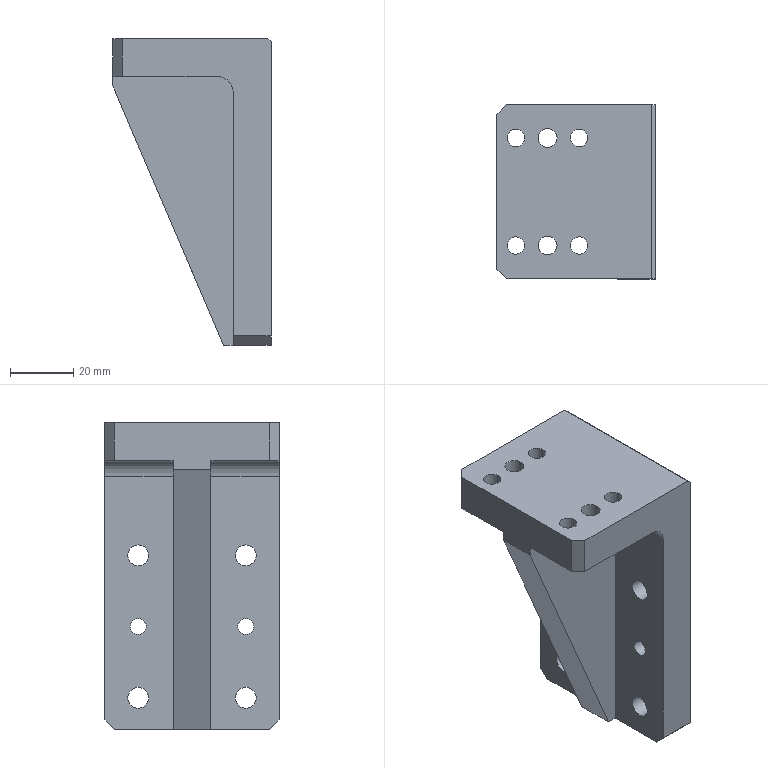Part | NX | 1 solid | 32 faces | box 50 x 55 x 97 mm | volume 106695 mm3 | plane 18 | cylinder 14 | commonest cylinder face diameters 5.5 x4 6.6 x4 5 x2 6 x2 10 x2
STEP:
#1=CARTESIAN_POINT('',(24.,55.,48.5));
#2=VERTEX_POINT('',#1);
#3=CARTESIAN_POINT('',(25.,55.,47.5));
#4=VERTEX_POINT('',#3);
#5=CARTESIAN_POINT('',(25.,55.,47.5));
#6=DIRECTION('',(0.7071,0.,-0.7071));
#7=VECTOR('',#6,1000.);
#8=LINE('',#5,#7);
#9=EDGE_CURVE('',#2,#4,#8,.T.);
#10=ORIENTED_EDGE('',*,*,#9,.F.);
#11=CARTESIAN_POINT('',(24.,0.,48.5));
#12=VERTEX_POINT('',#11);
#13=CARTESIAN_POINT('',(24.,55.,48.5));
#14=DIRECTION('',(0.,1.,0.));
#15=VECTOR('',#14,1000.);
#16=LINE('',#13,#15);
#17=EDGE_CURVE('',#12,#2,#16,.T.);
#18=ORIENTED_EDGE('',*,*,#17,.F.);
#19=CARTESIAN_POINT('',(25.,0.,47.5));
#20=VERTEX_POINT('',#19);
#21=CARTESIAN_POINT('',(36.25,0.,36.25));
#22=DIRECTION('',(-0.7071,0.,0.7071));
#23=VECTOR('',#22,1000.);
#24=LINE('',#21,#23);
#25=EDGE_CURVE('',#20,#12,#24,.T.);
#26=ORIENTED_EDGE('',*,*,#25,.F.);
#27=CARTESIAN_POINT('',(25.,55.,47.5));
#28=DIRECTION('',(0.,-1.,0.));
#29=VECTOR('',#28,1000.);
#30=LINE('',#27,#29);
#31=EDGE_CURVE('',#4,#20,#30,.T.);
#32=ORIENTED_EDGE('',*,*,#31,.F.);
#33=EDGE_LOOP('',(#10,#18,#26,#32));
#34=FACE_BOUND('',#33,.T.);
#35=CARTESIAN_POINT('',(25.,55.,47.5));
#36=DIRECTION('',(-0.7071,0.,-0.7071));
#37=DIRECTION('',(0.,-1.,0.));
#38=AXIS2_PLACEMENT_3D('',#35,#36,#37);
#39=PLANE('',#38);
#40=ADVANCED_FACE('',(#34),#39,.F.);
#41=CARTESIAN_POINT('',(25.,52.,-48.5));
#42=VERTEX_POINT('',#41);
#43=CARTESIAN_POINT('',(25.,55.,-45.5));
#44=VERTEX_POINT('',#43);
#45=CARTESIAN_POINT('',(25.,55.,-45.5));
#46=DIRECTION('',(0.,0.7071,0.7071));
#47=VECTOR('',#46,1000.);
#48=LINE('',#45,#47);
#49=EDGE_CURVE('',#42,#44,#48,.T.);
#50=ORIENTED_EDGE('',*,*,#49,.F.);
#51=CARTESIAN_POINT('',(13.,52.,-48.5));
#52=VERTEX_POINT('',#51);
#53=CARTESIAN_POINT('',(-25.,52.,-48.5));
#54=DIRECTION('',(1.,0.,0.));
#55=VECTOR('',#54,1000.);
#56=LINE('',#53,#55);
#57=EDGE_CURVE('',#52,#42,#56,.T.);
#58=ORIENTED_EDGE('',*,*,#57,.F.);
#59=CARTESIAN_POINT('',(13.,55.,-45.5));
#60=VERTEX_POINT('',#59);
#61=CARTESIAN_POINT('',(13.,55.,-45.5));
#62=DIRECTION('',(0.,-0.7071,-0.7071));
#63=VECTOR('',#62,1000.);
#64=LINE('',#61,#63);
#65=EDGE_CURVE('',#60,#52,#64,.T.);
#66=ORIENTED_EDGE('',*,*,#65,.F.);
#67=CARTESIAN_POINT('',(0.,55.,-45.5));
#68=DIRECTION('',(-1.,0.,0.));
#69=VECTOR('',#68,1000.);
#70=LINE('',#67,#69);
#71=EDGE_CURVE('',#44,#60,#70,.T.);
#72=ORIENTED_EDGE('',*,*,#71,.F.);
#73=EDGE_LOOP('',(#50,#58,#66,#72));
#74=FACE_BOUND('',#73,.T.);
#75=CARTESIAN_POINT('',(0.,55.,-45.5));
#76=DIRECTION('',(0.,-0.7071,0.7071));
#77=DIRECTION('',(-1.,0.,0.));
#78=AXIS2_PLACEMENT_3D('',#75,#76,#77);
#79=PLANE('',#78);
#80=ADVANCED_FACE('',(#74),#79,.F.);
#81=CARTESIAN_POINT('',(-25.,52.,36.5));
#82=VERTEX_POINT('',#81);
#83=CARTESIAN_POINT('',(-22.,55.,36.5));
#84=VERTEX_POINT('',#83);
#85=CARTESIAN_POINT('',(-22.,55.,36.5));
#86=DIRECTION('',(0.7071,0.7071,0.));
#87=VECTOR('',#86,1000.);
#88=LINE('',#85,#87);
#89=EDGE_CURVE('',#82,#84,#88,.T.);
#90=ORIENTED_EDGE('',*,*,#89,.F.);
#91=CARTESIAN_POINT('',(-25.,52.,48.5));
#92=VERTEX_POINT('',#91);
#93=CARTESIAN_POINT('',(-25.,52.,48.5));
#94=DIRECTION('',(0.,0.,-1.));
#95=VECTOR('',#94,1000.);
#96=LINE('',#93,#95);
#97=EDGE_CURVE('',#92,#82,#96,.T.);
#98=ORIENTED_EDGE('',*,*,#97,.F.);
#99=CARTESIAN_POINT('',(-22.,55.,48.5));
#100=VERTEX_POINT('',#99);
#101=CARTESIAN_POINT('',(-22.,55.,48.5));
#102=DIRECTION('',(-0.7071,-0.7071,0.));
#103=VECTOR('',#102,1000.);
#104=LINE('',#101,#103);
#105=EDGE_CURVE('',#100,#92,#104,.T.);
#106=ORIENTED_EDGE('',*,*,#105,.F.);
#107=CARTESIAN_POINT('',(-22.,55.,0.));
#108=DIRECTION('',(0.,0.,1.));
#109=VECTOR('',#108,1000.);
#110=LINE('',#107,#109);
#111=EDGE_CURVE('',#84,#100,#110,.T.);
#112=ORIENTED_EDGE('',*,*,#111,.F.);
#113=EDGE_LOOP('',(#90,#98,#106,#112));
#114=FACE_BOUND('',#113,.T.);
#115=CARTESIAN_POINT('',(-22.,55.,0.));
#116=DIRECTION('',(0.7071,-0.7071,0.));
#117=DIRECTION('',(0.,0.,1.));
#118=AXIS2_PLACEMENT_3D('',#115,#116,#117);
#119=PLANE('',#118);
#120=ADVANCED_FACE('',(#114),#119,.F.);
#121=CARTESIAN_POINT('',(25.,0.,-45.5));
#122=VERTEX_POINT('',#121);
#123=CARTESIAN_POINT('',(25.,3.,-48.5));
#124=VERTEX_POINT('',#123);
#125=CARTESIAN_POINT('',(25.,3.,-48.5));
#126=DIRECTION('',(0.,0.7071,-0.7071));
#127=VECTOR('',#126,1000.);
#128=LINE('',#125,#127);
#129=EDGE_CURVE('',#122,#124,#128,.T.);
#130=ORIENTED_EDGE('',*,*,#129,.F.);
#131=CARTESIAN_POINT('',(13.,0.,-45.5));
#132=VERTEX_POINT('',#131);
#133=CARTESIAN_POINT('',(25.,0.,-45.5));
#134=DIRECTION('',(1.,0.,0.));
#135=VECTOR('',#134,1000.);
#136=LINE('',#133,#135);
#137=EDGE_CURVE('',#132,#122,#136,.T.);
#138=ORIENTED_EDGE('',*,*,#137,.F.);
#139=CARTESIAN_POINT('',(13.,3.,-48.5));
#140=VERTEX_POINT('',#139);
#141=CARTESIAN_POINT('',(13.,18.25,-63.75));
#142=DIRECTION('',(0.,-0.7071,0.7071));
#143=VECTOR('',#142,1000.);
#144=LINE('',#141,#143);
#145=EDGE_CURVE('',#140,#132,#144,.T.);
#146=ORIENTED_EDGE('',*,*,#145,.F.);
#147=CARTESIAN_POINT('',(13.,3.,-48.5));
#148=DIRECTION('',(-1.,0.,0.));
#149=VECTOR('',#148,1000.);
#150=LINE('',#147,#149);
#151=EDGE_CURVE('',#124,#140,#150,.T.);
#152=ORIENTED_EDGE('',*,*,#151,.F.);
#153=EDGE_LOOP('',(#130,#138,#146,#152));
#154=FACE_BOUND('',#153,.T.);
#155=CARTESIAN_POINT('',(-25.,3.,-48.5));
#156=DIRECTION('',(0.,-0.7071,-0.7071));
#157=DIRECTION('',(1.,0.,0.));
#158=AXIS2_PLACEMENT_3D('',#155,#156,#157);
#159=PLANE('',#158);
#160=ADVANCED_FACE('',(#154),#159,.T.);
#161=CARTESIAN_POINT('',(-22.,0.,36.5));
#162=VERTEX_POINT('',#161);
#163=CARTESIAN_POINT('',(-25.,3.,36.5));
#164=VERTEX_POINT('',#163);
#165=CARTESIAN_POINT('',(-21.25,-0.75,36.5));
#166=DIRECTION('',(-0.7071,0.7071,0.));
#167=VECTOR('',#166,1000.);
#168=LINE('',#165,#167);
#169=EDGE_CURVE('',#162,#164,#168,.T.);
#170=ORIENTED_EDGE('',*,*,#169,.F.);
#171=CARTESIAN_POINT('',(-22.,0.,48.5));
#172=VERTEX_POINT('',#171);
#173=CARTESIAN_POINT('',(-22.,0.,36.5));
#174=DIRECTION('',(0.,0.,-1.));
#175=VECTOR('',#174,1000.);
#176=LINE('',#173,#175);
#177=EDGE_CURVE('',#172,#162,#176,.T.);
#178=ORIENTED_EDGE('',*,*,#177,.F.);
#179=CARTESIAN_POINT('',(-25.,3.,48.5));
#180=VERTEX_POINT('',#179);
#181=CARTESIAN_POINT('',(-25.,3.,48.5));
#182=DIRECTION('',(0.7071,-0.7071,0.));
#183=VECTOR('',#182,1000.);
#184=LINE('',#181,#183);
#185=EDGE_CURVE('',#180,#172,#184,.T.);
#186=ORIENTED_EDGE('',*,*,#185,.F.);
#187=CARTESIAN_POINT('',(-25.,3.,48.5));
#188=DIRECTION('',(0.,0.,1.));
#189=VECTOR('',#188,1000.);
#190=LINE('',#187,#189);
#191=EDGE_CURVE('',#164,#180,#190,.T.);
#192=ORIENTED_EDGE('',*,*,#191,.F.);
#193=EDGE_LOOP('',(#170,#178,#186,#192));
#194=FACE_BOUND('',#193,.T.);
#195=CARTESIAN_POINT('',(-25.,3.,48.5));
#196=DIRECTION('',(-0.7071,-0.7071,0.));
#197=DIRECTION('',(0.,0.,-1.));
#198=AXIS2_PLACEMENT_3D('',#195,#196,#197);
#199=PLANE('',#198);
#200=ADVANCED_FACE('',(#194),#199,.T.);
#201=CARTESIAN_POINT('',(8.,33.5,36.5));
#202=VERTEX_POINT('',#201);
#203=CARTESIAN_POINT('',(13.,33.5,31.5));
#204=VERTEX_POINT('',#203);
#205=CARTESIAN_POINT('',(8.,33.5,31.5));
#206=DIRECTION('',(0.,1.,0.));
#207=DIRECTION('',(0.,0.,1.));
#208=AXIS2_PLACEMENT_3D('',#205,#206,#207);
#209=CIRCLE('',#208,5.);
#210=EDGE_CURVE('',#202,#204,#209,.T.);
#211=ORIENTED_EDGE('',*,*,#210,.F.);
#212=CARTESIAN_POINT('',(8.,55.,36.5));
#213=VERTEX_POINT('',#212);
#214=CARTESIAN_POINT('',(8.,33.5,36.5));
#215=DIRECTION('',(0.,-1.,0.));
#216=VECTOR('',#215,1000.);
#217=LINE('',#214,#216);
#218=EDGE_CURVE('',#213,#202,#217,.T.);
#219=ORIENTED_EDGE('',*,*,#218,.F.);
#220=CARTESIAN_POINT('',(13.,55.,31.5));
#221=VERTEX_POINT('',#220);
#222=CARTESIAN_POINT('',(8.,55.,31.5));
#223=DIRECTION('',(0.,-1.,0.));
#224=DIRECTION('',(0.,0.,-1.));
#225=AXIS2_PLACEMENT_3D('',#222,#223,#224);
#226=CIRCLE('',#225,5.);
#227=EDGE_CURVE('',#221,#213,#226,.T.);
#228=ORIENTED_EDGE('',*,*,#227,.F.);
#229=CARTESIAN_POINT('',(13.,55.,31.5));
#230=DIRECTION('',(0.,1.,0.));
#231=VECTOR('',#230,1000.);
#232=LINE('',#229,#231);
#233=EDGE_CURVE('',#204,#221,#232,.T.);
#234=ORIENTED_EDGE('',*,*,#233,.F.);
#235=EDGE_LOOP('',(#211,#219,#228,#234));
#236=FACE_BOUND('',#235,.T.);
#237=CARTESIAN_POINT('',(8.,33.5,31.5));
#238=DIRECTION('',(0.,-1.,0.));
#239=DIRECTION('',(0.,0.,-1.));
#240=AXIS2_PLACEMENT_3D('',#237,#238,#239);
#241=CYLINDRICAL_SURFACE('',#240,5.);
#242=ADVANCED_FACE('',(#236),#241,.F.);
#243=CARTESIAN_POINT('',(13.,21.5,31.5));
#244=VERTEX_POINT('',#243);
#245=CARTESIAN_POINT('',(8.,21.5,36.5));
#246=VERTEX_POINT('',#245);
#247=CARTESIAN_POINT('',(8.,21.5,31.5));
#248=DIRECTION('',(0.,-1.,0.));
#249=DIRECTION('',(0.,0.,-1.));
#250=AXIS2_PLACEMENT_3D('',#247,#248,#249);
#251=CIRCLE('',#250,5.);
#252=EDGE_CURVE('',#244,#246,#251,.T.);
#253=ORIENTED_EDGE('',*,*,#252,.F.);
#254=CARTESIAN_POINT('',(13.,0.,31.5));
#255=VERTEX_POINT('',#254);
#256=CARTESIAN_POINT('',(13.,21.5,31.5));
#257=DIRECTION('',(0.,1.,0.));
#258=VECTOR('',#257,1000.);
#259=LINE('',#256,#258);
#260=EDGE_CURVE('',#255,#244,#259,.T.);
#261=ORIENTED_EDGE('',*,*,#260,.F.);
#262=CARTESIAN_POINT('',(8.,0.,36.5));
#263=VERTEX_POINT('',#262);
#264=CARTESIAN_POINT('',(8.,0.,31.5));
#265=DIRECTION('',(0.,1.,0.));
#266=DIRECTION('',(0.,0.,-1.));
#267=AXIS2_PLACEMENT_3D('',#264,#265,#266);
#268=CIRCLE('',#267,5.);
#269=EDGE_CURVE('',#263,#255,#268,.T.);
#270=ORIENTED_EDGE('',*,*,#269,.F.);
#271=CARTESIAN_POINT('',(8.,21.5,36.5));
#272=DIRECTION('',(0.,-1.,0.));
#273=VECTOR('',#272,1000.);
#274=LINE('',#271,#273);
#275=EDGE_CURVE('',#246,#263,#274,.T.);
#276=ORIENTED_EDGE('',*,*,#275,.F.);
#277=EDGE_LOOP('',(#253,#261,#270,#276));
#278=FACE_BOUND('',#277,.T.);
#279=CARTESIAN_POINT('',(8.,21.5,31.5));
#280=DIRECTION('',(0.,1.,0.));
#281=DIRECTION('',(0.,0.,1.));
#282=AXIS2_PLACEMENT_3D('',#279,#280,#281);
#283=CYLINDRICAL_SURFACE('',#282,5.);
#284=ADVANCED_FACE('',(#278),#283,.F.);
#285=CARTESIAN_POINT('',(13.,21.5,-48.5));
#286=VERTEX_POINT('',#285);
#287=CARTESIAN_POINT('',(13.,21.5,-48.5));
#288=DIRECTION('',(0.,0.,-1.));
#289=VECTOR('',#288,1000.);
#290=LINE('',#287,#289);
#291=EDGE_CURVE('',#244,#286,#290,.T.);
#292=ORIENTED_EDGE('',*,*,#291,.F.);
#293=ORIENTED_EDGE('',*,*,#252,.T.);
#294=CARTESIAN_POINT('',(-25.,21.5,36.5));
#295=VERTEX_POINT('',#294);
#296=CARTESIAN_POINT('',(13.,21.5,36.5));
#297=DIRECTION('',(1.,0.,0.));
#298=VECTOR('',#297,1000.);
#299=LINE('',#296,#298);
#300=EDGE_CURVE('',#295,#246,#299,.T.);
#301=ORIENTED_EDGE('',*,*,#300,.F.);
#302=CARTESIAN_POINT('',(-25.,21.5,33.5));
#303=VERTEX_POINT('',#302);
#304=CARTESIAN_POINT('',(-25.,21.5,33.5));
#305=DIRECTION('',(0.,0.,1.));
#306=VECTOR('',#305,1000.);
#307=LINE('',#304,#306);
#308=EDGE_CURVE('',#303,#295,#307,.T.);
#309=ORIENTED_EDGE('',*,*,#308,.F.);
#310=CARTESIAN_POINT('',(10.,21.5,-48.5));
#311=VERTEX_POINT('',#310);
#312=CARTESIAN_POINT('',(-25.,21.5,33.5));
#313=DIRECTION('',(-0.3926,0.,0.9197));
#314=VECTOR('',#313,1000.);
#315=LINE('',#312,#314);
#316=EDGE_CURVE('',#311,#303,#315,.T.);
#317=ORIENTED_EDGE('',*,*,#316,.F.);
#318=CARTESIAN_POINT('',(13.,21.5,-48.5));
#319=DIRECTION('',(-1.,0.,0.));
#320=VECTOR('',#319,1000.);
#321=LINE('',#318,#320);
#322=EDGE_CURVE('',#286,#311,#321,.T.);
#323=ORIENTED_EDGE('',*,*,#322,.F.);
#324=EDGE_LOOP('',(#292,#293,#301,#309,#317,#323));
#325=FACE_BOUND('',#324,.T.);
#326=CARTESIAN_POINT('',(0.,21.5,0.));
#327=DIRECTION('',(0.,-1.,0.));
#328=DIRECTION('',(0.,0.,1.));
#329=AXIS2_PLACEMENT_3D('',#326,#327,#328);
#330=PLANE('',#329);
#331=ADVANCED_FACE('',(#325),#330,.T.);
#332=CARTESIAN_POINT('',(13.,33.5,-48.5));
#333=DIRECTION('',(0.,-1.,0.));
#334=VECTOR('',#333,1000.);
#335=LINE('',#332,#334);
#336=EDGE_CURVE('',#286,#140,#335,.T.);
#337=ORIENTED_EDGE('',*,*,#336,.T.);
#338=ORIENTED_EDGE('',*,*,#145,.T.);
#339=CARTESIAN_POINT('',(13.,0.,0.));
#340=DIRECTION('',(0.,0.,-1.));
#341=VECTOR('',#340,1000.);
#342=LINE('',#339,#341);
#343=EDGE_CURVE('',#255,#132,#342,.T.);
#344=ORIENTED_EDGE('',*,*,#343,.F.);
#345=ORIENTED_EDGE('',*,*,#260,.T.);
#346=ORIENTED_EDGE('',*,*,#291,.T.);
#347=EDGE_LOOP('',(#337,#338,#344,#345,#346));
#348=FACE_BOUND('',#347,.T.);
#349=CARTESIAN_POINT('',(13.,10.5,3.2));
#350=VERTEX_POINT('',#349);
#351=CARTESIAN_POINT('',(13.,10.5,6.5));
#352=DIRECTION('',(-1.,0.,0.));
#353=DIRECTION('',(0.,0.,-1.));
#354=AXIS2_PLACEMENT_3D('',#351,#352,#353);
#355=CIRCLE('',#354,3.3);
#356=EDGE_CURVE('',#350,#350,#355,.T.);
#357=ORIENTED_EDGE('',*,*,#356,.F.);
#358=EDGE_LOOP('',(#357));
#359=FACE_BOUND('',#358,.T.);
#360=CARTESIAN_POINT('',(13.,10.5,-41.8));
#361=VERTEX_POINT('',#360);
#362=CARTESIAN_POINT('',(13.,10.5,-38.5));
#363=DIRECTION('',(-1.,0.,0.));
#364=DIRECTION('',(0.,0.,-1.));
#365=AXIS2_PLACEMENT_3D('',#362,#363,#364);
#366=CIRCLE('',#365,3.3);
#367=EDGE_CURVE('',#361,#361,#366,.T.);
#368=ORIENTED_EDGE('',*,*,#367,.F.);
#369=EDGE_LOOP('',(#368));
#370=FACE_BOUND('',#369,.T.);
#371=CARTESIAN_POINT('',(13.,10.5,-18.5));
#372=VERTEX_POINT('',#371);
#373=CARTESIAN_POINT('',(13.,10.5,-16.));
#374=DIRECTION('',(-1.,0.,0.));
#375=DIRECTION('',(0.,0.,-1.));
#376=AXIS2_PLACEMENT_3D('',#373,#374,#375);
#377=CIRCLE('',#376,2.5);
#378=EDGE_CURVE('',#372,#372,#377,.T.);
#379=ORIENTED_EDGE('',*,*,#378,.F.);
#380=EDGE_LOOP('',(#379));
#381=FACE_BOUND('',#380,.T.);
#382=CARTESIAN_POINT('',(13.,33.5,-48.5));
#383=DIRECTION('',(1.,0.,0.));
#384=DIRECTION('',(0.,0.,-1.));
#385=AXIS2_PLACEMENT_3D('',#382,#383,#384);
#386=PLANE('',#385);
#387=ADVANCED_FACE('',(#348,#359,#370,#381),#386,.F.);
#388=CARTESIAN_POINT('',(0.,0.,36.5));
#389=DIRECTION('',(1.,0.,0.));
#390=VECTOR('',#389,1000.);
#391=LINE('',#388,#390);
#392=EDGE_CURVE('',#162,#263,#391,.T.);
#393=ORIENTED_EDGE('',*,*,#392,.F.);
#394=ORIENTED_EDGE('',*,*,#169,.T.);
#395=CARTESIAN_POINT('',(-25.,55.,36.5));
#396=DIRECTION('',(0.,-1.,0.));
#397=VECTOR('',#396,1000.);
#398=LINE('',#395,#397);
#399=EDGE_CURVE('',#295,#164,#398,.T.);
#400=ORIENTED_EDGE('',*,*,#399,.F.);
#401=ORIENTED_EDGE('',*,*,#300,.T.);
#402=ORIENTED_EDGE('',*,*,#275,.T.);
#403=EDGE_LOOP('',(#393,#394,#400,#401,#402));
#404=FACE_BOUND('',#403,.T.);
#405=CARTESIAN_POINT('',(-16.25,10.5,36.5));
#406=VERTEX_POINT('',#405);
#407=CARTESIAN_POINT('',(-19.,10.5,36.5));
#408=DIRECTION('',(0.,0.,-1.));
#409=DIRECTION('',(1.,0.,0.));
#410=AXIS2_PLACEMENT_3D('',#407,#408,#409);
#411=CIRCLE('',#410,2.75);
#412=EDGE_CURVE('',#406,#406,#411,.T.);
#413=ORIENTED_EDGE('',*,*,#412,.F.);
#414=EDGE_LOOP('',(#413));
#415=FACE_BOUND('',#414,.T.);
#416=CARTESIAN_POINT('',(3.75,10.5,36.5));
#417=VERTEX_POINT('',#416);
#418=CARTESIAN_POINT('',(1.,10.5,36.5));
#419=DIRECTION('',(0.,0.,-1.));
#420=DIRECTION('',(1.,0.,0.));
#421=AXIS2_PLACEMENT_3D('',#418,#419,#420);
#422=CIRCLE('',#421,2.75);
#423=EDGE_CURVE('',#417,#417,#422,.T.);
#424=ORIENTED_EDGE('',*,*,#423,.F.);
#425=EDGE_LOOP('',(#424));
#426=FACE_BOUND('',#425,.T.);
#427=CARTESIAN_POINT('',(-6.,10.5,36.5));
#428=VERTEX_POINT('',#427);
#429=CARTESIAN_POINT('',(-9.,10.5,36.5));
#430=DIRECTION('',(0.,0.,-1.));
#431=DIRECTION('',(1.,0.,0.));
#432=AXIS2_PLACEMENT_3D('',#429,#430,#431);
#433=CIRCLE('',#432,3.);
#434=EDGE_CURVE('',#428,#428,#433,.T.);
#435=ORIENTED_EDGE('',*,*,#434,.F.);
#436=EDGE_LOOP('',(#435));
#437=FACE_BOUND('',#436,.T.);
#438=CARTESIAN_POINT('',(13.,33.5,36.5));
#439=DIRECTION('',(0.,0.,1.));
#440=DIRECTION('',(1.,0.,0.));
#441=AXIS2_PLACEMENT_3D('',#438,#439,#440);
#442=PLANE('',#441);
#443=ADVANCED_FACE('',(#404,#415,#426,#437),#442,.F.);
#444=CARTESIAN_POINT('',(-25.,33.5,36.5));
#445=VERTEX_POINT('',#444);
#446=CARTESIAN_POINT('',(13.,33.5,36.5));
#447=DIRECTION('',(1.,0.,0.));
#448=VECTOR('',#447,1000.);
#449=LINE('',#446,#448);
#450=EDGE_CURVE('',#445,#202,#449,.T.);
#451=ORIENTED_EDGE('',*,*,#450,.T.);
#452=ORIENTED_EDGE('',*,*,#210,.T.);
#453=CARTESIAN_POINT('',(13.,33.5,-48.5));
#454=VERTEX_POINT('',#453);
#455=CARTESIAN_POINT('',(13.,33.5,-48.5));
#456=DIRECTION('',(0.,0.,-1.));
#457=VECTOR('',#456,1000.);
#458=LINE('',#455,#457);
#459=EDGE_CURVE('',#204,#454,#458,.T.);
#460=ORIENTED_EDGE('',*,*,#459,.T.);
#461=CARTESIAN_POINT('',(10.,33.5,-48.5));
#462=VERTEX_POINT('',#461);
#463=CARTESIAN_POINT('',(13.,33.5,-48.5));
#464=DIRECTION('',(-1.,0.,0.));
#465=VECTOR('',#464,1000.);
#466=LINE('',#463,#465);
#467=EDGE_CURVE('',#454,#462,#466,.T.);
#468=ORIENTED_EDGE('',*,*,#467,.T.);
#469=CARTESIAN_POINT('',(-25.,33.5,33.5));
#470=VERTEX_POINT('',#469);
#471=CARTESIAN_POINT('',(-25.,33.5,33.5));
#472=DIRECTION('',(-0.3926,0.,0.9197));
#473=VECTOR('',#472,1000.);
#474=LINE('',#471,#473);
#475=EDGE_CURVE('',#462,#470,#474,.T.);
#476=ORIENTED_EDGE('',*,*,#475,.T.);
#477=CARTESIAN_POINT('',(-25.,33.5,33.5));
#478=DIRECTION('',(0.,0.,1.));
#479=VECTOR('',#478,1000.);
#480=LINE('',#477,#479);
#481=EDGE_CURVE('',#470,#445,#480,.T.);
#482=ORIENTED_EDGE('',*,*,#481,.T.);
#483=EDGE_LOOP('',(#451,#452,#460,#468,#476,#482));
#484=FACE_BOUND('',#483,.T.);
#485=CARTESIAN_POINT('',(0.,33.5,0.));
#486=DIRECTION('',(0.,1.,0.));
#487=DIRECTION('',(0.,0.,1.));
#488=AXIS2_PLACEMENT_3D('',#485,#486,#487);
#489=PLANE('',#488);
#490=ADVANCED_FACE('',(#484),#489,.T.);
#491=CARTESIAN_POINT('',(-25.,33.5,36.5));
#492=DIRECTION('',(0.,1.,0.));
#493=VECTOR('',#492,1000.);
#494=LINE('',#491,#493);
#495=EDGE_CURVE('',#445,#82,#494,.T.);
#496=ORIENTED_EDGE('',*,*,#495,.T.);
#497=ORIENTED_EDGE('',*,*,#89,.T.);
#498=CARTESIAN_POINT('',(13.,55.,36.5));
#499=DIRECTION('',(1.,0.,0.));
#500=VECTOR('',#499,1000.);
#501=LINE('',#498,#500);
#502=EDGE_CURVE('',#84,#213,#501,.T.);
#503=ORIENTED_EDGE('',*,*,#502,.T.);
#504=ORIENTED_EDGE('',*,*,#218,.T.);
#505=ORIENTED_EDGE('',*,*,#450,.F.);
#506=EDGE_LOOP('',(#496,#497,#503,#504,#505));
#507=FACE_BOUND('',#506,.T.);
#508=CARTESIAN_POINT('',(-21.75,44.5,36.5));
#509=VERTEX_POINT('',#508);
#510=CARTESIAN_POINT('',(-19.,44.5,36.5));
#511=DIRECTION('',(0.,0.,-1.));
#512=DIRECTION('',(-1.,0.,0.));
#513=AXIS2_PLACEMENT_3D('',#510,#511,#512);
#514=CIRCLE('',#513,2.75);
#515=EDGE_CURVE('',#509,#509,#514,.T.);
#516=ORIENTED_EDGE('',*,*,#515,.F.);
#517=EDGE_LOOP('',(#516));
#518=FACE_BOUND('',#517,.T.);
#519=CARTESIAN_POINT('',(-1.75,44.5,36.5));
#520=VERTEX_POINT('',#519);
#521=CARTESIAN_POINT('',(1.,44.5,36.5));
#522=DIRECTION('',(0.,0.,-1.));
#523=DIRECTION('',(-1.,0.,0.));
#524=AXIS2_PLACEMENT_3D('',#521,#522,#523);
#525=CIRCLE('',#524,2.75);
#526=EDGE_CURVE('',#520,#520,#525,.T.);
#527=ORIENTED_EDGE('',*,*,#526,.F.);
#528=EDGE_LOOP('',(#527));
#529=FACE_BOUND('',#528,.T.);
#530=CARTESIAN_POINT('',(-12.,44.5,36.5));
#531=VERTEX_POINT('',#530);
#532=CARTESIAN_POINT('',(-9.,44.5,36.5));
#533=DIRECTION('',(0.,0.,-1.));
#534=DIRECTION('',(-1.,0.,0.));
#535=AXIS2_PLACEMENT_3D('',#532,#533,#534);
#536=CIRCLE('',#535,3.);
#537=EDGE_CURVE('',#531,#531,#536,.T.);
#538=ORIENTED_EDGE('',*,*,#537,.F.);
#539=EDGE_LOOP('',(#538));
#540=FACE_BOUND('',#539,.T.);
#541=CARTESIAN_POINT('',(13.,33.5,36.5));
#542=DIRECTION('',(0.,0.,1.));
#543=DIRECTION('',(1.,0.,0.));
#544=AXIS2_PLACEMENT_3D('',#541,#542,#543);
#545=PLANE('',#544);
#546=ADVANCED_FACE('',(#507,#518,#529,#540),#545,.F.);
#547=CARTESIAN_POINT('',(13.,55.,-48.5));
#548=DIRECTION('',(0.,0.,-1.));
#549=VECTOR('',#548,1000.);
#550=LINE('',#547,#549);
#551=EDGE_CURVE('',#221,#60,#550,.T.);
#552=ORIENTED_EDGE('',*,*,#551,.T.);
#553=ORIENTED_EDGE('',*,*,#65,.T.);
#554=CARTESIAN_POINT('',(13.,33.5,-48.5));
#555=DIRECTION('',(0.,1.,0.));
#556=VECTOR('',#555,1000.);
#557=LINE('',#554,#556);
#558=EDGE_CURVE('',#454,#52,#557,.T.);
#559=ORIENTED_EDGE('',*,*,#558,.F.);
#560=ORIENTED_EDGE('',*,*,#459,.F.);
#561=ORIENTED_EDGE('',*,*,#233,.T.);
#562=EDGE_LOOP('',(#552,#553,#559,#560,#561));
#563=FACE_BOUND('',#562,.T.);
#564=CARTESIAN_POINT('',(13.,44.5,9.8));
#565=VERTEX_POINT('',#564);
#566=CARTESIAN_POINT('',(13.,44.5,6.5));
#567=DIRECTION('',(-1.,0.,0.));
#568=DIRECTION('',(0.,0.,1.));
#569=AXIS2_PLACEMENT_3D('',#566,#567,#568);
#570=CIRCLE('',#569,3.3);
#571=EDGE_CURVE('',#565,#565,#570,.T.);
#572=ORIENTED_EDGE('',*,*,#571,.F.);
#573=EDGE_LOOP('',(#572));
#574=FACE_BOUND('',#573,.T.);
#575=CARTESIAN_POINT('',(13.,44.5,-35.2));
#576=VERTEX_POINT('',#575);
#577=CARTESIAN_POINT('',(13.,44.5,-38.5));
#578=DIRECTION('',(-1.,0.,0.));
#579=DIRECTION('',(0.,0.,1.));
#580=AXIS2_PLACEMENT_3D('',#577,#578,#579);
#581=CIRCLE('',#580,3.3);
#582=EDGE_CURVE('',#576,#576,#581,.T.);
#583=ORIENTED_EDGE('',*,*,#582,.F.);
#584=EDGE_LOOP('',(#583));
#585=FACE_BOUND('',#584,.T.);
#586=CARTESIAN_POINT('',(13.,44.5,-13.5));
#587=VERTEX_POINT('',#586);
#588=CARTESIAN_POINT('',(13.,44.5,-16.));
#589=DIRECTION('',(-1.,0.,0.));
#590=DIRECTION('',(0.,0.,1.));
#591=AXIS2_PLACEMENT_3D('',#588,#589,#590);
#592=CIRCLE('',#591,2.5);
#593=EDGE_CURVE('',#587,#587,#592,.T.);
#594=ORIENTED_EDGE('',*,*,#593,.F.);
#595=EDGE_LOOP('',(#594));
#596=FACE_BOUND('',#595,.T.);
#597=CARTESIAN_POINT('',(13.,33.5,-48.5));
#598=DIRECTION('',(1.,0.,0.));
#599=DIRECTION('',(0.,0.,-1.));
#600=AXIS2_PLACEMENT_3D('',#597,#598,#599);
#601=PLANE('',#600);
#602=ADVANCED_FACE('',(#563,#574,#585,#596),#601,.F.);
#603=CARTESIAN_POINT('',(-25.,55.,48.5));
#604=DIRECTION('',(1.,0.,0.));
#605=VECTOR('',#604,1000.);
#606=LINE('',#603,#605);
#607=EDGE_CURVE('',#100,#2,#606,.T.);
#608=ORIENTED_EDGE('',*,*,#607,.T.);
#609=ORIENTED_EDGE('',*,*,#9,.T.);
#610=CARTESIAN_POINT('',(25.,55.,48.5));
#611=DIRECTION('',(0.,0.,-1.));
#612=VECTOR('',#611,1000.);
#613=LINE('',#610,#612);
#614=EDGE_CURVE('',#4,#44,#613,.T.);
#615=ORIENTED_EDGE('',*,*,#614,.T.);
#616=ORIENTED_EDGE('',*,*,#71,.T.);
#617=ORIENTED_EDGE('',*,*,#551,.F.);
#618=ORIENTED_EDGE('',*,*,#227,.T.);
#619=ORIENTED_EDGE('',*,*,#502,.F.);
#620=ORIENTED_EDGE('',*,*,#111,.T.);
#621=EDGE_LOOP('',(#608,#609,#615,#616,#617,#618,#619,#620));
#622=FACE_BOUND('',#621,.T.);
#623=CARTESIAN_POINT('',(0.,55.,0.));
#624=DIRECTION('',(0.,-1.,0.));
#625=DIRECTION('',(0.,0.,-1.));
#626=AXIS2_PLACEMENT_3D('',#623,#624,#625);
#627=PLANE('',#626);
#628=ADVANCED_FACE('',(#622),#627,.F.);
#629=CARTESIAN_POINT('',(-25.,0.,48.5));
#630=DIRECTION('',(1.,0.,0.));
#631=VECTOR('',#630,1000.);
#632=LINE('',#629,#631);
#633=EDGE_CURVE('',#172,#12,#632,.T.);
#634=ORIENTED_EDGE('',*,*,#633,.T.);
#635=ORIENTED_EDGE('',*,*,#17,.T.);
#636=ORIENTED_EDGE('',*,*,#607,.F.);
#637=ORIENTED_EDGE('',*,*,#105,.T.);
#638=CARTESIAN_POINT('',(-25.,55.,48.5));
#639=DIRECTION('',(0.,-1.,0.));
#640=VECTOR('',#639,1000.);
#641=LINE('',#638,#640);
#642=EDGE_CURVE('',#92,#180,#641,.T.);
#643=ORIENTED_EDGE('',*,*,#642,.T.);
#644=ORIENTED_EDGE('',*,*,#185,.T.);
#645=EDGE_LOOP('',(#634,#635,#636,#637,#643,#644));
#646=FACE_BOUND('',#645,.T.);
#647=CARTESIAN_POINT('',(-21.75,44.5,48.5));
#648=VERTEX_POINT('',#647);
#649=CARTESIAN_POINT('',(-19.,44.5,48.5));
#650=DIRECTION('',(0.,0.,-1.));
#651=DIRECTION('',(-1.,0.,0.));
#652=AXIS2_PLACEMENT_3D('',#649,#650,#651);
#653=CIRCLE('',#652,2.75);
#654=EDGE_CURVE('',#648,#648,#653,.T.);
#655=ORIENTED_EDGE('',*,*,#654,.T.);
#656=EDGE_LOOP('',(#655));
#657=FACE_BOUND('',#656,.T.);
#658=CARTESIAN_POINT('',(-1.75,44.5,48.5));
#659=VERTEX_POINT('',#658);
#660=CARTESIAN_POINT('',(1.,44.5,48.5));
#661=DIRECTION('',(0.,0.,-1.));
#662=DIRECTION('',(-1.,0.,0.));
#663=AXIS2_PLACEMENT_3D('',#660,#661,#662);
#664=CIRCLE('',#663,2.75);
#665=EDGE_CURVE('',#659,#659,#664,.T.);
#666=ORIENTED_EDGE('',*,*,#665,.T.);
#667=EDGE_LOOP('',(#666));
#668=FACE_BOUND('',#667,.T.);
#669=CARTESIAN_POINT('',(-21.75,10.5,48.5));
#670=VERTEX_POINT('',#669);
#671=CARTESIAN_POINT('',(-19.,10.5,48.5));
#672=DIRECTION('',(0.,0.,-1.));
#673=DIRECTION('',(-1.,0.,0.));
#674=AXIS2_PLACEMENT_3D('',#671,#672,#673);
#675=CIRCLE('',#674,2.75);
#676=EDGE_CURVE('',#670,#670,#675,.T.);
#677=ORIENTED_EDGE('',*,*,#676,.T.);
#678=EDGE_LOOP('',(#677));
#679=FACE_BOUND('',#678,.T.);
#680=CARTESIAN_POINT('',(-1.75,10.5,48.5));
#681=VERTEX_POINT('',#680);
#682=CARTESIAN_POINT('',(1.,10.5,48.5));
#683=DIRECTION('',(0.,0.,-1.));
#684=DIRECTION('',(-1.,0.,0.));
#685=AXIS2_PLACEMENT_3D('',#682,#683,#684);
#686=CIRCLE('',#685,2.75);
#687=EDGE_CURVE('',#681,#681,#686,.T.);
#688=ORIENTED_EDGE('',*,*,#687,.T.);
#689=EDGE_LOOP('',(#688));
#690=FACE_BOUND('',#689,.T.);
#691=CARTESIAN_POINT('',(-12.,44.5,48.5));
#692=VERTEX_POINT('',#691);
#693=CARTESIAN_POINT('',(-9.,44.5,48.5));
#694=DIRECTION('',(0.,0.,-1.));
#695=DIRECTION('',(-1.,0.,0.));
#696=AXIS2_PLACEMENT_3D('',#693,#694,#695);
#697=CIRCLE('',#696,3.);
#698=EDGE_CURVE('',#692,#692,#697,.T.);
#699=ORIENTED_EDGE('',*,*,#698,.T.);
#700=EDGE_LOOP('',(#699));
#701=FACE_BOUND('',#700,.T.);
#702=CARTESIAN_POINT('',(-12.,10.5,48.5));
#703=VERTEX_POINT('',#702);
#704=CARTESIAN_POINT('',(-9.,10.5,48.5));
#705=DIRECTION('',(0.,0.,-1.));
#706=DIRECTION('',(-1.,0.,0.));
#707=AXIS2_PLACEMENT_3D('',#704,#705,#706);
#708=CIRCLE('',#707,3.);
#709=EDGE_CURVE('',#703,#703,#708,.T.);
#710=ORIENTED_EDGE('',*,*,#709,.T.);
#711=EDGE_LOOP('',(#710));
#712=FACE_BOUND('',#711,.T.);
#713=CARTESIAN_POINT('',(-25.,55.,48.5));
#714=DIRECTION('',(0.,0.,-1.));
#715=DIRECTION('',(-1.,0.,0.));
#716=AXIS2_PLACEMENT_3D('',#713,#714,#715);
#717=PLANE('',#716);
#718=ADVANCED_FACE('',(#646,#657,#668,#679,#690,#701,#712),#717,.F.);
#719=ORIENTED_EDGE('',*,*,#614,.F.);
#720=ORIENTED_EDGE('',*,*,#31,.T.);
#721=CARTESIAN_POINT('',(25.,0.,48.5));
#722=DIRECTION('',(0.,0.,-1.));
#723=VECTOR('',#722,1000.);
#724=LINE('',#721,#723);
#725=EDGE_CURVE('',#20,#122,#724,.T.);
#726=ORIENTED_EDGE('',*,*,#725,.T.);
#727=ORIENTED_EDGE('',*,*,#129,.T.);
#728=CARTESIAN_POINT('',(25.,55.,-48.5));
#729=DIRECTION('',(0.,-1.,0.));
#730=VECTOR('',#729,1000.);
#731=LINE('',#728,#730);
#732=EDGE_CURVE('',#42,#124,#731,.T.);
#733=ORIENTED_EDGE('',*,*,#732,.F.);
#734=ORIENTED_EDGE('',*,*,#49,.T.);
#735=EDGE_LOOP('',(#719,#720,#726,#727,#733,#734));
#736=FACE_BOUND('',#735,.T.);
#737=CARTESIAN_POINT('',(25.,44.5,9.8));
#738=VERTEX_POINT('',#737);
#739=CARTESIAN_POINT('',(25.,44.5,6.5));
#740=DIRECTION('',(-1.,0.,0.));
#741=DIRECTION('',(0.,0.,1.));
#742=AXIS2_PLACEMENT_3D('',#739,#740,#741);
#743=CIRCLE('',#742,3.3);
#744=EDGE_CURVE('',#738,#738,#743,.T.);
#745=ORIENTED_EDGE('',*,*,#744,.T.);
#746=EDGE_LOOP('',(#745));
#747=FACE_BOUND('',#746,.T.);
#748=CARTESIAN_POINT('',(25.,10.5,9.8));
#749=VERTEX_POINT('',#748);
#750=CARTESIAN_POINT('',(25.,10.5,6.5));
#751=DIRECTION('',(-1.,0.,0.));
#752=DIRECTION('',(0.,0.,1.));
#753=AXIS2_PLACEMENT_3D('',#750,#751,#752);
#754=CIRCLE('',#753,3.3);
#755=EDGE_CURVE('',#749,#749,#754,.T.);
#756=ORIENTED_EDGE('',*,*,#755,.T.);
#757=EDGE_LOOP('',(#756));
#758=FACE_BOUND('',#757,.T.);
#759=CARTESIAN_POINT('',(25.,44.5,-35.2));
#760=VERTEX_POINT('',#759);
#761=CARTESIAN_POINT('',(25.,44.5,-38.5));
#762=DIRECTION('',(-1.,0.,0.));
#763=DIRECTION('',(0.,0.,1.));
#764=AXIS2_PLACEMENT_3D('',#761,#762,#763);
#765=CIRCLE('',#764,3.3);
#766=EDGE_CURVE('',#760,#760,#765,.T.);
#767=ORIENTED_EDGE('',*,*,#766,.T.);
#768=EDGE_LOOP('',(#767));
#769=FACE_BOUND('',#768,.T.);
#770=CARTESIAN_POINT('',(25.,10.5,-35.2));
#771=VERTEX_POINT('',#770);
#772=CARTESIAN_POINT('',(25.,10.5,-38.5));
#773=DIRECTION('',(-1.,0.,0.));
#774=DIRECTION('',(0.,0.,1.));
#775=AXIS2_PLACEMENT_3D('',#772,#773,#774);
#776=CIRCLE('',#775,3.3);
#777=EDGE_CURVE('',#771,#771,#776,.T.);
#778=ORIENTED_EDGE('',*,*,#777,.T.);
#779=EDGE_LOOP('',(#778));
#780=FACE_BOUND('',#779,.T.);
#781=CARTESIAN_POINT('',(25.,44.5,-13.5));
#782=VERTEX_POINT('',#781);
#783=CARTESIAN_POINT('',(25.,44.5,-16.));
#784=DIRECTION('',(-1.,0.,0.));
#785=DIRECTION('',(0.,0.,1.));
#786=AXIS2_PLACEMENT_3D('',#783,#784,#785);
#787=CIRCLE('',#786,2.5);
#788=EDGE_CURVE('',#782,#782,#787,.T.);
#789=ORIENTED_EDGE('',*,*,#788,.T.);
#790=EDGE_LOOP('',(#789));
#791=FACE_BOUND('',#790,.T.);
#792=CARTESIAN_POINT('',(25.,10.5,-13.5));
#793=VERTEX_POINT('',#792);
#794=CARTESIAN_POINT('',(25.,10.5,-16.));
#795=DIRECTION('',(-1.,0.,0.));
#796=DIRECTION('',(0.,0.,1.));
#797=AXIS2_PLACEMENT_3D('',#794,#795,#796);
#798=CIRCLE('',#797,2.5);
#799=EDGE_CURVE('',#793,#793,#798,.T.);
#800=ORIENTED_EDGE('',*,*,#799,.T.);
#801=EDGE_LOOP('',(#800));
#802=FACE_BOUND('',#801,.T.);
#803=CARTESIAN_POINT('',(25.,55.,48.5));
#804=DIRECTION('',(-1.,0.,0.));
#805=DIRECTION('',(0.,0.,1.));
#806=AXIS2_PLACEMENT_3D('',#803,#804,#805);
#807=PLANE('',#806);
#808=ADVANCED_FACE('',(#736,#747,#758,#769,#780,#791,#802),#807,.F.);
#809=ORIENTED_EDGE('',*,*,#725,.F.);
#810=ORIENTED_EDGE('',*,*,#25,.T.);
#811=ORIENTED_EDGE('',*,*,#633,.F.);
#812=ORIENTED_EDGE('',*,*,#177,.T.);
#813=ORIENTED_EDGE('',*,*,#392,.T.);
#814=ORIENTED_EDGE('',*,*,#269,.T.);
#815=ORIENTED_EDGE('',*,*,#343,.T.);
#816=ORIENTED_EDGE('',*,*,#137,.T.);
#817=EDGE_LOOP('',(#809,#810,#811,#812,#813,#814,#815,#816));
#818=FACE_BOUND('',#817,.T.);
#819=CARTESIAN_POINT('',(0.,0.,0.));
#820=DIRECTION('',(0.,-1.,0.));
#821=DIRECTION('',(0.,0.,-1.));
#822=AXIS2_PLACEMENT_3D('',#819,#820,#821);
#823=PLANE('',#822);
#824=ADVANCED_FACE('',(#818),#823,.T.);
#825=ORIENTED_EDGE('',*,*,#399,.T.);
#826=ORIENTED_EDGE('',*,*,#191,.T.);
#827=ORIENTED_EDGE('',*,*,#642,.F.);
#828=ORIENTED_EDGE('',*,*,#97,.T.);
#829=ORIENTED_EDGE('',*,*,#495,.F.);
#830=ORIENTED_EDGE('',*,*,#481,.F.);
#831=CARTESIAN_POINT('',(-25.,0.,33.5));
#832=DIRECTION('',(0.,1.,0.));
#833=VECTOR('',#832,1000.);
#834=LINE('',#831,#833);
#835=EDGE_CURVE('',#303,#470,#834,.T.);
#836=ORIENTED_EDGE('',*,*,#835,.F.);
#837=ORIENTED_EDGE('',*,*,#308,.T.);
#838=EDGE_LOOP('',(#825,#826,#827,#828,#829,#830,#836,#837));
#839=FACE_BOUND('',#838,.T.);
#840=CARTESIAN_POINT('',(-25.,55.,48.5));
#841=DIRECTION('',(1.,0.,0.));
#842=DIRECTION('',(0.,0.,-1.));
#843=AXIS2_PLACEMENT_3D('',#840,#841,#842);
#844=PLANE('',#843);
#845=ADVANCED_FACE('',(#839),#844,.F.);
#846=ORIENTED_EDGE('',*,*,#732,.T.);
#847=ORIENTED_EDGE('',*,*,#151,.T.);
#848=ORIENTED_EDGE('',*,*,#336,.F.);
#849=ORIENTED_EDGE('',*,*,#322,.T.);
#850=CARTESIAN_POINT('',(10.,0.,-48.5));
#851=DIRECTION('',(0.,1.,0.));
#852=VECTOR('',#851,1000.);
#853=LINE('',#850,#852);
#854=EDGE_CURVE('',#311,#462,#853,.T.);
#855=ORIENTED_EDGE('',*,*,#854,.T.);
#856=ORIENTED_EDGE('',*,*,#467,.F.);
#857=ORIENTED_EDGE('',*,*,#558,.T.);
#858=ORIENTED_EDGE('',*,*,#57,.T.);
#859=EDGE_LOOP('',(#846,#847,#848,#849,#855,#856,#857,#858));
#860=FACE_BOUND('',#859,.T.);
#861=CARTESIAN_POINT('',(-25.,55.,-48.5));
#862=DIRECTION('',(0.,0.,1.));
#863=DIRECTION('',(1.,0.,0.));
#864=AXIS2_PLACEMENT_3D('',#861,#862,#863);
#865=PLANE('',#864);
#866=ADVANCED_FACE('',(#860),#865,.F.);
#867=ORIENTED_EDGE('',*,*,#316,.T.);
#868=ORIENTED_EDGE('',*,*,#835,.T.);
#869=ORIENTED_EDGE('',*,*,#475,.F.);
#870=ORIENTED_EDGE('',*,*,#854,.F.);
#871=EDGE_LOOP('',(#867,#868,#869,#870));
#872=FACE_BOUND('',#871,.T.);
#873=CARTESIAN_POINT('',(10.,0.,-48.5));
#874=DIRECTION('',(0.9197,0.,0.3926));
#875=DIRECTION('',(0.3926,0.,-0.9197));
#876=AXIS2_PLACEMENT_3D('',#873,#874,#875);
#877=PLANE('',#876);
#878=ADVANCED_FACE('',(#872),#877,.F.);
#879=ORIENTED_EDGE('',*,*,#515,.T.);
#880=EDGE_LOOP('',(#879));
#881=FACE_BOUND('',#880,.T.);
#882=ORIENTED_EDGE('',*,*,#654,.F.);
#883=EDGE_LOOP('',(#882));
#884=FACE_BOUND('',#883,.T.);
#885=CARTESIAN_POINT('',(-19.,44.5,36.5));
#886=DIRECTION('',(0.,0.,-1.));
#887=DIRECTION('',(-1.,0.,0.));
#888=AXIS2_PLACEMENT_3D('',#885,#886,#887);
#889=CYLINDRICAL_SURFACE('',#888,2.75);
#890=ADVANCED_FACE('',(#881,#884),#889,.F.);
#891=ORIENTED_EDGE('',*,*,#526,.T.);
#892=EDGE_LOOP('',(#891));
#893=FACE_BOUND('',#892,.T.);
#894=ORIENTED_EDGE('',*,*,#665,.F.);
#895=EDGE_LOOP('',(#894));
#896=FACE_BOUND('',#895,.T.);
#897=CARTESIAN_POINT('',(1.,44.5,36.5));
#898=DIRECTION('',(0.,0.,-1.));
#899=DIRECTION('',(-1.,0.,0.));
#900=AXIS2_PLACEMENT_3D('',#897,#898,#899);
#901=CYLINDRICAL_SURFACE('',#900,2.75);
#902=ADVANCED_FACE('',(#893,#896),#901,.F.);
#903=ORIENTED_EDGE('',*,*,#412,.T.);
#904=EDGE_LOOP('',(#903));
#905=FACE_BOUND('',#904,.T.);
#906=ORIENTED_EDGE('',*,*,#676,.F.);
#907=EDGE_LOOP('',(#906));
#908=FACE_BOUND('',#907,.T.);
#909=CARTESIAN_POINT('',(-19.,10.5,36.5));
#910=DIRECTION('',(0.,0.,-1.));
#911=DIRECTION('',(-1.,0.,0.));
#912=AXIS2_PLACEMENT_3D('',#909,#910,#911);
#913=CYLINDRICAL_SURFACE('',#912,2.75);
#914=ADVANCED_FACE('',(#905,#908),#913,.F.);
#915=ORIENTED_EDGE('',*,*,#423,.T.);
#916=EDGE_LOOP('',(#915));
#917=FACE_BOUND('',#916,.T.);
#918=ORIENTED_EDGE('',*,*,#687,.F.);
#919=EDGE_LOOP('',(#918));
#920=FACE_BOUND('',#919,.T.);
#921=CARTESIAN_POINT('',(1.,10.5,36.5));
#922=DIRECTION('',(0.,0.,-1.));
#923=DIRECTION('',(-1.,0.,0.));
#924=AXIS2_PLACEMENT_3D('',#921,#922,#923);
#925=CYLINDRICAL_SURFACE('',#924,2.75);
#926=ADVANCED_FACE('',(#917,#920),#925,.F.);
#927=ORIENTED_EDGE('',*,*,#744,.F.);
#928=EDGE_LOOP('',(#927));
#929=FACE_BOUND('',#928,.T.);
#930=ORIENTED_EDGE('',*,*,#571,.T.);
#931=EDGE_LOOP('',(#930));
#932=FACE_BOUND('',#931,.T.);
#933=CARTESIAN_POINT('',(13.,44.5,6.5));
#934=DIRECTION('',(-1.,0.,0.));
#935=DIRECTION('',(0.,0.,1.));
#936=AXIS2_PLACEMENT_3D('',#933,#934,#935);
#937=CYLINDRICAL_SURFACE('',#936,3.3);
#938=ADVANCED_FACE('',(#929,#932),#937,.F.);
#939=ORIENTED_EDGE('',*,*,#755,.F.);
#940=EDGE_LOOP('',(#939));
#941=FACE_BOUND('',#940,.T.);
#942=ORIENTED_EDGE('',*,*,#356,.T.);
#943=EDGE_LOOP('',(#942));
#944=FACE_BOUND('',#943,.T.);
#945=CARTESIAN_POINT('',(13.,10.5,6.5));
#946=DIRECTION('',(-1.,0.,0.));
#947=DIRECTION('',(0.,0.,1.));
#948=AXIS2_PLACEMENT_3D('',#945,#946,#947);
#949=CYLINDRICAL_SURFACE('',#948,3.3);
#950=ADVANCED_FACE('',(#941,#944),#949,.F.);
#951=ORIENTED_EDGE('',*,*,#766,.F.);
#952=EDGE_LOOP('',(#951));
#953=FACE_BOUND('',#952,.T.);
#954=ORIENTED_EDGE('',*,*,#582,.T.);
#955=EDGE_LOOP('',(#954));
#956=FACE_BOUND('',#955,.T.);
#957=CARTESIAN_POINT('',(13.,44.5,-38.5));
#958=DIRECTION('',(-1.,0.,0.));
#959=DIRECTION('',(0.,0.,1.));
#960=AXIS2_PLACEMENT_3D('',#957,#958,#959);
#961=CYLINDRICAL_SURFACE('',#960,3.3);
#962=ADVANCED_FACE('',(#953,#956),#961,.F.);
#963=ORIENTED_EDGE('',*,*,#777,.F.);
#964=EDGE_LOOP('',(#963));
#965=FACE_BOUND('',#964,.T.);
#966=ORIENTED_EDGE('',*,*,#367,.T.);
#967=EDGE_LOOP('',(#966));
#968=FACE_BOUND('',#967,.T.);
#969=CARTESIAN_POINT('',(13.,10.5,-38.5));
#970=DIRECTION('',(-1.,0.,0.));
#971=DIRECTION('',(0.,0.,1.));
#972=AXIS2_PLACEMENT_3D('',#969,#970,#971);
#973=CYLINDRICAL_SURFACE('',#972,3.3);
#974=ADVANCED_FACE('',(#965,#968),#973,.F.);
#975=ORIENTED_EDGE('',*,*,#537,.T.);
#976=EDGE_LOOP('',(#975));
#977=FACE_BOUND('',#976,.T.);
#978=ORIENTED_EDGE('',*,*,#698,.F.);
#979=EDGE_LOOP('',(#978));
#980=FACE_BOUND('',#979,.T.);
#981=CARTESIAN_POINT('',(-9.,44.5,36.5));
#982=DIRECTION('',(0.,0.,-1.));
#983=DIRECTION('',(-1.,0.,0.));
#984=AXIS2_PLACEMENT_3D('',#981,#982,#983);
#985=CYLINDRICAL_SURFACE('',#984,3.);
#986=ADVANCED_FACE('',(#977,#980),#985,.F.);
#987=ORIENTED_EDGE('',*,*,#434,.T.);
#988=EDGE_LOOP('',(#987));
#989=FACE_BOUND('',#988,.T.);
#990=ORIENTED_EDGE('',*,*,#709,.F.);
#991=EDGE_LOOP('',(#990));
#992=FACE_BOUND('',#991,.T.);
#993=CARTESIAN_POINT('',(-9.,10.5,36.5));
#994=DIRECTION('',(0.,0.,-1.));
#995=DIRECTION('',(-1.,0.,0.));
#996=AXIS2_PLACEMENT_3D('',#993,#994,#995);
#997=CYLINDRICAL_SURFACE('',#996,3.);
#998=ADVANCED_FACE('',(#989,#992),#997,.F.);
#999=ORIENTED_EDGE('',*,*,#788,.F.);
#1000=EDGE_LOOP('',(#999));
#1001=FACE_BOUND('',#1000,.T.);
#1002=ORIENTED_EDGE('',*,*,#593,.T.);
#1003=EDGE_LOOP('',(#1002));
#1004=FACE_BOUND('',#1003,.T.);
#1005=CARTESIAN_POINT('',(13.,44.5,-16.));
#1006=DIRECTION('',(-1.,0.,0.));
#1007=DIRECTION('',(0.,0.,1.));
#1008=AXIS2_PLACEMENT_3D('',#1005,#1006,#1007);
#1009=CYLINDRICAL_SURFACE('',#1008,2.5);
#1010=ADVANCED_FACE('',(#1001,#1004),#1009,.F.);
#1011=ORIENTED_EDGE('',*,*,#799,.F.);
#1012=EDGE_LOOP('',(#1011));
#1013=FACE_BOUND('',#1012,.T.);
#1014=ORIENTED_EDGE('',*,*,#378,.T.);
#1015=EDGE_LOOP('',(#1014));
#1016=FACE_BOUND('',#1015,.T.);
#1017=CARTESIAN_POINT('',(13.,10.5,-16.));
#1018=DIRECTION('',(-1.,0.,0.));
#1019=DIRECTION('',(0.,0.,1.));
#1020=AXIS2_PLACEMENT_3D('',#1017,#1018,#1019);
#1021=CYLINDRICAL_SURFACE('',#1020,2.5);
#1022=ADVANCED_FACE('',(#1013,#1016),#1021,.F.);
#1023=CLOSED_SHELL('',(#40,#80,#120,#160,#200,#242,#284,#331,#387,#443,#490,#546,#602,#628,#718,#808,#824,#845,#866,#878,#890,#902,#914,#926,#938,#950,#962,#974,#986,#998,#1010,#1022));
#1024=MANIFOLD_SOLID_BREP('',#1023);
#1025=(LENGTH_UNIT()NAMED_UNIT(*)SI_UNIT(.MILLI.,.METRE.));
#1026=UNCERTAINTY_MEASURE_WITH_UNIT(LENGTH_MEASURE(0.00001),#1025,'','');
#1027=(NAMED_UNIT(*)PLANE_ANGLE_UNIT()SI_UNIT($,.RADIAN.));
#1028=(NAMED_UNIT(*)SI_UNIT($,.STERADIAN.)SOLID_ANGLE_UNIT());
#1029=(GEOMETRIC_REPRESENTATION_CONTEXT(3)GLOBAL_UNCERTAINTY_ASSIGNED_CONTEXT((#1026))GLOBAL_UNIT_ASSIGNED_CONTEXT((#1025,#1027,#1028))REPRESENTATION_CONTEXT('',''));
#1030=ADVANCED_BREP_SHAPE_REPRESENTATION('',(#1024),#1029);